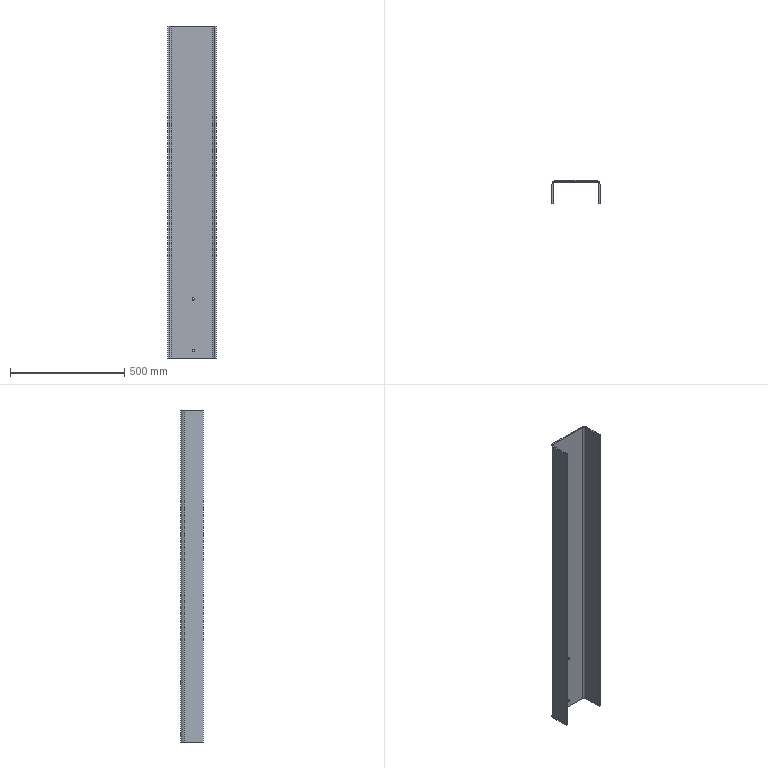Part | STEP file | _20001 | 1 solid | 18 faces | box 210 x 100 x 1450 mm | volume 3332053 mm3 | plane 10 | cylinder 8 | commonest cylinder face diameters 10.8 x4 18 x2 34 x2
STEP:
#1=CARTESIAN_POINT('',(10.9,0.,-467.));
#2=VERTEX_POINT('',#1);
#3=CARTESIAN_POINT('',(10.9,-6.,-467.));
#4=VERTEX_POINT('',#3);
#5=CARTESIAN_POINT('',(10.9,0.,-467.));
#6=DIRECTION('',(0.,-1.,0.));
#7=VECTOR('',#6,1000.);
#8=LINE('',#5,#7);
#9=EDGE_CURVE('',#2,#4,#8,.T.);
#10=ORIENTED_EDGE('',*,*,#9,.F.);
#11=CARTESIAN_POINT('',(0.1,0.,-467.));
#12=VERTEX_POINT('',#11);
#13=CARTESIAN_POINT('',(5.5,0.,-467.));
#14=DIRECTION('',(0.,-1.,0.));
#15=DIRECTION('',(-1.,0.,0.));
#16=AXIS2_PLACEMENT_3D('',#13,#14,#15);
#17=CIRCLE('',#16,5.4);
#18=EDGE_CURVE('',#12,#2,#17,.T.);
#19=ORIENTED_EDGE('',*,*,#18,.F.);
#20=CARTESIAN_POINT('',(0.1,-6.,-467.));
#21=VERTEX_POINT('',#20);
#22=CARTESIAN_POINT('',(0.1,0.,-467.));
#23=DIRECTION('',(0.,-1.,0.));
#24=VECTOR('',#23,1000.);
#25=LINE('',#22,#24);
#26=EDGE_CURVE('',#12,#21,#25,.T.);
#27=ORIENTED_EDGE('',*,*,#26,.T.);
#28=CARTESIAN_POINT('',(5.5,-6.,-467.));
#29=DIRECTION('',(0.,1.,0.));
#30=DIRECTION('',(1.,0.,0.));
#31=AXIS2_PLACEMENT_3D('',#28,#29,#30);
#32=CIRCLE('',#31,5.4);
#33=EDGE_CURVE('',#4,#21,#32,.T.);
#34=ORIENTED_EDGE('',*,*,#33,.F.);
#35=EDGE_LOOP('',(#10,#19,#27,#34));
#36=FACE_OUTER_BOUND('',#35,.T.);
#37=CARTESIAN_POINT('',(5.5,-10.,-467.));
#38=DIRECTION('',(0.,1.,0.));
#39=DIRECTION('',(-1.,0.,0.));
#40=AXIS2_PLACEMENT_3D('',#37,#38,#39);
#41=CYLINDRICAL_SURFACE('',#40,5.4);
#42=ADVANCED_FACE('',(#36),#41,.F.);
#43=CARTESIAN_POINT('',(5.5,-6.,-467.));
#44=DIRECTION('',(0.,1.,0.));
#45=DIRECTION('',(-1.,0.,0.));
#46=AXIS2_PLACEMENT_3D('',#43,#44,#45);
#47=CIRCLE('',#46,5.4);
#48=EDGE_CURVE('',#21,#4,#47,.T.);
#49=ORIENTED_EDGE('',*,*,#48,.F.);
#50=ORIENTED_EDGE('',*,*,#26,.F.);
#51=CARTESIAN_POINT('',(5.5,0.,-467.));
#52=DIRECTION('',(0.,-1.,0.));
#53=DIRECTION('',(1.,0.,0.));
#54=AXIS2_PLACEMENT_3D('',#51,#52,#53);
#55=CIRCLE('',#54,5.4);
#56=EDGE_CURVE('',#2,#12,#55,.T.);
#57=ORIENTED_EDGE('',*,*,#56,.F.);
#58=ORIENTED_EDGE('',*,*,#9,.T.);
#59=EDGE_LOOP('',(#49,#50,#57,#58));
#60=FACE_OUTER_BOUND('',#59,.T.);
#61=CARTESIAN_POINT('',(5.5,-10.,-467.));
#62=DIRECTION('',(0.,1.,0.));
#63=DIRECTION('',(-1.,0.,0.));
#64=AXIS2_PLACEMENT_3D('',#61,#62,#63);
#65=CYLINDRICAL_SURFACE('',#64,5.4);
#66=ADVANCED_FACE('',(#60),#65,.F.);
#67=CARTESIAN_POINT('',(88.,0.,-725.));
#68=VERTEX_POINT('',#67);
#69=CARTESIAN_POINT('',(88.,0.,725.));
#70=VERTEX_POINT('',#69);
#71=CARTESIAN_POINT('',(88.,0.,-725.));
#72=DIRECTION('',(0.,0.,1.));
#73=VECTOR('',#72,1000.);
#74=LINE('',#71,#73);
#75=EDGE_CURVE('',#68,#70,#74,.T.);
#76=ORIENTED_EDGE('',*,*,#75,.T.);
#77=CARTESIAN_POINT('',(105.,-17.,725.));
#78=VERTEX_POINT('',#77);
#79=CARTESIAN_POINT('',(88.,-17.,725.));
#80=DIRECTION('',(0.,0.,1.));
#81=DIRECTION('',(1.,0.,0.));
#82=AXIS2_PLACEMENT_3D('',#79,#80,#81);
#83=CIRCLE('',#82,17.);
#84=EDGE_CURVE('',#78,#70,#83,.T.);
#85=ORIENTED_EDGE('',*,*,#84,.F.);
#86=CARTESIAN_POINT('',(105.,-17.,-725.));
#87=VERTEX_POINT('',#86);
#88=CARTESIAN_POINT('',(105.,-17.,725.));
#89=DIRECTION('',(0.,0.,-1.));
#90=VECTOR('',#89,1000.);
#91=LINE('',#88,#90);
#92=EDGE_CURVE('',#78,#87,#91,.T.);
#93=ORIENTED_EDGE('',*,*,#92,.T.);
#94=CARTESIAN_POINT('',(88.,-17.,-725.));
#95=DIRECTION('',(0.,0.,-1.));
#96=DIRECTION('',(0.,1.,0.));
#97=AXIS2_PLACEMENT_3D('',#94,#95,#96);
#98=CIRCLE('',#97,17.);
#99=EDGE_CURVE('',#68,#87,#98,.T.);
#100=ORIENTED_EDGE('',*,*,#99,.F.);
#101=EDGE_LOOP('',(#76,#85,#93,#100));
#102=FACE_OUTER_BOUND('',#101,.T.);
#103=CARTESIAN_POINT('',(88.,-17.,725.));
#104=DIRECTION('',(0.,0.,-1.));
#105=DIRECTION('',(-1.,0.,0.));
#106=AXIS2_PLACEMENT_3D('',#103,#104,#105);
#107=CYLINDRICAL_SURFACE('',#106,17.);
#108=ADVANCED_FACE('',(#102),#107,.T.);
#109=ORIENTED_EDGE('',*,*,#92,.F.);
#110=CARTESIAN_POINT('',(105.,-100.,725.));
#111=VERTEX_POINT('',#110);
#112=CARTESIAN_POINT('',(105.,-17.,725.));
#113=DIRECTION('',(0.,-1.,0.));
#114=VECTOR('',#113,1000.);
#115=LINE('',#112,#114);
#116=EDGE_CURVE('',#78,#111,#115,.T.);
#117=ORIENTED_EDGE('',*,*,#116,.T.);
#118=CARTESIAN_POINT('',(105.,-100.,-725.));
#119=VERTEX_POINT('',#118);
#120=CARTESIAN_POINT('',(105.,-100.,-725.));
#121=DIRECTION('',(0.,0.,1.));
#122=VECTOR('',#121,1000.);
#123=LINE('',#120,#122);
#124=EDGE_CURVE('',#119,#111,#123,.T.);
#125=ORIENTED_EDGE('',*,*,#124,.F.);
#126=CARTESIAN_POINT('',(105.,-17.,-725.));
#127=DIRECTION('',(0.,-1.,0.));
#128=VECTOR('',#127,1000.);
#129=LINE('',#126,#128);
#130=EDGE_CURVE('',#87,#119,#129,.T.);
#131=ORIENTED_EDGE('',*,*,#130,.F.);
#132=EDGE_LOOP('',(#109,#117,#125,#131));
#133=FACE_OUTER_BOUND('',#132,.T.);
#134=CARTESIAN_POINT('',(105.,0.,725.));
#135=DIRECTION('',(-1.,0.,0.));
#136=DIRECTION('',(0.,0.,1.));
#137=AXIS2_PLACEMENT_3D('',#134,#135,#136);
#138=PLANE('',#137);
#139=ADVANCED_FACE('',(#133),#138,.F.);
#140=ORIENTED_EDGE('',*,*,#124,.T.);
#141=CARTESIAN_POINT('',(99.,-100.,725.));
#142=VERTEX_POINT('',#141);
#143=CARTESIAN_POINT('',(99.,-100.,725.));
#144=DIRECTION('',(1.,0.,0.));
#145=VECTOR('',#144,1000.);
#146=LINE('',#143,#145);
#147=EDGE_CURVE('',#142,#111,#146,.T.);
#148=ORIENTED_EDGE('',*,*,#147,.F.);
#149=CARTESIAN_POINT('',(99.,-100.,-725.));
#150=VERTEX_POINT('',#149);
#151=CARTESIAN_POINT('',(99.,-100.,-725.));
#152=DIRECTION('',(0.,0.,1.));
#153=VECTOR('',#152,1000.);
#154=LINE('',#151,#153);
#155=EDGE_CURVE('',#150,#142,#154,.T.);
#156=ORIENTED_EDGE('',*,*,#155,.F.);
#157=CARTESIAN_POINT('',(99.,-100.,-725.));
#158=DIRECTION('',(1.,0.,0.));
#159=VECTOR('',#158,1000.);
#160=LINE('',#157,#159);
#161=EDGE_CURVE('',#150,#119,#160,.T.);
#162=ORIENTED_EDGE('',*,*,#161,.T.);
#163=EDGE_LOOP('',(#140,#148,#156,#162));
#164=FACE_OUTER_BOUND('',#163,.T.);
#165=CARTESIAN_POINT('',(105.,-100.,725.));
#166=DIRECTION('',(0.,-1.,0.));
#167=DIRECTION('',(0.,0.,-1.));
#168=AXIS2_PLACEMENT_3D('',#165,#166,#167);
#169=PLANE('',#168);
#170=ADVANCED_FACE('',(#164),#169,.T.);
#171=CARTESIAN_POINT('',(99.,-15.,-725.));
#172=VERTEX_POINT('',#171);
#173=CARTESIAN_POINT('',(99.,-15.,-725.));
#174=DIRECTION('',(0.,-1.,0.));
#175=VECTOR('',#174,1000.);
#176=LINE('',#173,#175);
#177=EDGE_CURVE('',#172,#150,#176,.T.);
#178=ORIENTED_EDGE('',*,*,#177,.T.);
#179=ORIENTED_EDGE('',*,*,#155,.T.);
#180=CARTESIAN_POINT('',(99.,-15.,725.));
#181=VERTEX_POINT('',#180);
#182=CARTESIAN_POINT('',(99.,-100.,725.));
#183=DIRECTION('',(0.,1.,0.));
#184=VECTOR('',#183,1000.);
#185=LINE('',#182,#184);
#186=EDGE_CURVE('',#142,#181,#185,.T.);
#187=ORIENTED_EDGE('',*,*,#186,.T.);
#188=CARTESIAN_POINT('',(99.,-15.,-725.));
#189=DIRECTION('',(0.,0.,1.));
#190=VECTOR('',#189,1000.);
#191=LINE('',#188,#190);
#192=EDGE_CURVE('',#172,#181,#191,.T.);
#193=ORIENTED_EDGE('',*,*,#192,.F.);
#194=EDGE_LOOP('',(#178,#179,#187,#193));
#195=FACE_OUTER_BOUND('',#194,.T.);
#196=CARTESIAN_POINT('',(99.,0.,725.));
#197=DIRECTION('',(-1.,0.,0.));
#198=DIRECTION('',(0.,0.,1.));
#199=AXIS2_PLACEMENT_3D('',#196,#197,#198);
#200=PLANE('',#199);
#201=ADVANCED_FACE('',(#195),#200,.T.);
#202=CARTESIAN_POINT('',(90.,-6.,-725.));
#203=VERTEX_POINT('',#202);
#204=CARTESIAN_POINT('',(90.,-15.,-725.));
#205=DIRECTION('',(0.,0.,1.));
#206=DIRECTION('',(1.,0.,0.));
#207=AXIS2_PLACEMENT_3D('',#204,#205,#206);
#208=CIRCLE('',#207,9.);
#209=EDGE_CURVE('',#172,#203,#208,.T.);
#210=ORIENTED_EDGE('',*,*,#209,.F.);
#211=ORIENTED_EDGE('',*,*,#192,.T.);
#212=CARTESIAN_POINT('',(90.,-6.,725.));
#213=VERTEX_POINT('',#212);
#214=CARTESIAN_POINT('',(90.,-15.,725.));
#215=DIRECTION('',(0.,0.,-1.));
#216=DIRECTION('',(0.,1.,0.));
#217=AXIS2_PLACEMENT_3D('',#214,#215,#216);
#218=CIRCLE('',#217,9.);
#219=EDGE_CURVE('',#213,#181,#218,.T.);
#220=ORIENTED_EDGE('',*,*,#219,.F.);
#221=CARTESIAN_POINT('',(90.,-6.,-725.));
#222=DIRECTION('',(0.,0.,1.));
#223=VECTOR('',#222,1000.);
#224=LINE('',#221,#223);
#225=EDGE_CURVE('',#203,#213,#224,.T.);
#226=ORIENTED_EDGE('',*,*,#225,.F.);
#227=EDGE_LOOP('',(#210,#211,#220,#226));
#228=FACE_OUTER_BOUND('',#227,.T.);
#229=CARTESIAN_POINT('',(90.,-15.,-2615.22));
#230=DIRECTION('',(0.,0.,1.));
#231=DIRECTION('',(1.,0.,0.));
#232=AXIS2_PLACEMENT_3D('',#229,#230,#231);
#233=CYLINDRICAL_SURFACE('',#232,9.);
#234=ADVANCED_FACE('',(#228),#233,.F.);
#235=CARTESIAN_POINT('',(-105.,-17.,-725.));
#236=VERTEX_POINT('',#235);
#237=CARTESIAN_POINT('',(-105.,-17.,725.));
#238=VERTEX_POINT('',#237);
#239=CARTESIAN_POINT('',(-105.,-17.,-725.));
#240=DIRECTION('',(0.,0.,1.));
#241=VECTOR('',#240,1000.);
#242=LINE('',#239,#241);
#243=EDGE_CURVE('',#236,#238,#242,.T.);
#244=ORIENTED_EDGE('',*,*,#243,.T.);
#245=CARTESIAN_POINT('',(-88.,0.,725.));
#246=VERTEX_POINT('',#245);
#247=CARTESIAN_POINT('',(-88.,-17.,725.));
#248=DIRECTION('',(0.,0.,1.));
#249=DIRECTION('',(0.,1.,0.));
#250=AXIS2_PLACEMENT_3D('',#247,#248,#249);
#251=CIRCLE('',#250,17.);
#252=EDGE_CURVE('',#246,#238,#251,.T.);
#253=ORIENTED_EDGE('',*,*,#252,.F.);
#254=CARTESIAN_POINT('',(-88.,0.,-725.));
#255=VERTEX_POINT('',#254);
#256=CARTESIAN_POINT('',(-88.,0.,725.));
#257=DIRECTION('',(0.,0.,-1.));
#258=VECTOR('',#257,1000.);
#259=LINE('',#256,#258);
#260=EDGE_CURVE('',#246,#255,#259,.T.);
#261=ORIENTED_EDGE('',*,*,#260,.T.);
#262=CARTESIAN_POINT('',(-88.,-17.,-725.));
#263=DIRECTION('',(0.,0.,-1.));
#264=DIRECTION('',(-1.,0.,0.));
#265=AXIS2_PLACEMENT_3D('',#262,#263,#264);
#266=CIRCLE('',#265,17.);
#267=EDGE_CURVE('',#236,#255,#266,.T.);
#268=ORIENTED_EDGE('',*,*,#267,.F.);
#269=EDGE_LOOP('',(#244,#253,#261,#268));
#270=FACE_OUTER_BOUND('',#269,.T.);
#271=CARTESIAN_POINT('',(-88.,-17.,725.));
#272=DIRECTION('',(0.,0.,-1.));
#273=DIRECTION('',(-1.,0.,0.));
#274=AXIS2_PLACEMENT_3D('',#271,#272,#273);
#275=CYLINDRICAL_SURFACE('',#274,17.);
#276=ADVANCED_FACE('',(#270),#275,.T.);
#277=CARTESIAN_POINT('',(-105.,-100.,-725.));
#278=VERTEX_POINT('',#277);
#279=CARTESIAN_POINT('',(-105.,-100.,725.));
#280=VERTEX_POINT('',#279);
#281=CARTESIAN_POINT('',(-105.,-100.,-725.));
#282=DIRECTION('',(0.,0.,1.));
#283=VECTOR('',#282,1000.);
#284=LINE('',#281,#283);
#285=EDGE_CURVE('',#278,#280,#284,.T.);
#286=ORIENTED_EDGE('',*,*,#285,.T.);
#287=CARTESIAN_POINT('',(-105.,-100.,725.));
#288=DIRECTION('',(0.,1.,0.));
#289=VECTOR('',#288,1000.);
#290=LINE('',#287,#289);
#291=EDGE_CURVE('',#280,#238,#290,.T.);
#292=ORIENTED_EDGE('',*,*,#291,.T.);
#293=ORIENTED_EDGE('',*,*,#243,.F.);
#294=CARTESIAN_POINT('',(-105.,-100.,-725.));
#295=DIRECTION('',(0.,1.,0.));
#296=VECTOR('',#295,1000.);
#297=LINE('',#294,#296);
#298=EDGE_CURVE('',#278,#236,#297,.T.);
#299=ORIENTED_EDGE('',*,*,#298,.F.);
#300=EDGE_LOOP('',(#286,#292,#293,#299));
#301=FACE_OUTER_BOUND('',#300,.T.);
#302=CARTESIAN_POINT('',(-105.,0.,725.));
#303=DIRECTION('',(1.,0.,0.));
#304=DIRECTION('',(0.,1.,0.));
#305=AXIS2_PLACEMENT_3D('',#302,#303,#304);
#306=PLANE('',#305);
#307=ADVANCED_FACE('',(#301),#306,.F.);
#308=CARTESIAN_POINT('',(-99.,-100.,-725.));
#309=VERTEX_POINT('',#308);
#310=CARTESIAN_POINT('',(-99.,-100.,725.));
#311=VERTEX_POINT('',#310);
#312=CARTESIAN_POINT('',(-99.,-100.,-725.));
#313=DIRECTION('',(0.,0.,1.));
#314=VECTOR('',#313,1000.);
#315=LINE('',#312,#314);
#316=EDGE_CURVE('',#309,#311,#315,.T.);
#317=ORIENTED_EDGE('',*,*,#316,.T.);
#318=CARTESIAN_POINT('',(-105.,-100.,725.));
#319=DIRECTION('',(1.,0.,0.));
#320=VECTOR('',#319,1000.);
#321=LINE('',#318,#320);
#322=EDGE_CURVE('',#280,#311,#321,.T.);
#323=ORIENTED_EDGE('',*,*,#322,.F.);
#324=ORIENTED_EDGE('',*,*,#285,.F.);
#325=CARTESIAN_POINT('',(-105.,-100.,-725.));
#326=DIRECTION('',(1.,0.,0.));
#327=VECTOR('',#326,1000.);
#328=LINE('',#325,#327);
#329=EDGE_CURVE('',#278,#309,#328,.T.);
#330=ORIENTED_EDGE('',*,*,#329,.T.);
#331=EDGE_LOOP('',(#317,#323,#324,#330));
#332=FACE_OUTER_BOUND('',#331,.T.);
#333=CARTESIAN_POINT('',(-97.,-100.,725.));
#334=DIRECTION('',(0.,-1.,0.));
#335=DIRECTION('',(0.,0.,-1.));
#336=AXIS2_PLACEMENT_3D('',#333,#334,#335);
#337=PLANE('',#336);
#338=ADVANCED_FACE('',(#332),#337,.T.);
#339=CARTESIAN_POINT('',(-90.,-6.,-725.));
#340=VERTEX_POINT('',#339);
#341=CARTESIAN_POINT('',(-99.,-15.,-725.));
#342=VERTEX_POINT('',#341);
#343=CARTESIAN_POINT('',(-90.,-15.,-725.));
#344=DIRECTION('',(0.,0.,1.));
#345=DIRECTION('',(0.,1.,0.));
#346=AXIS2_PLACEMENT_3D('',#343,#344,#345);
#347=CIRCLE('',#346,9.);
#348=EDGE_CURVE('',#340,#342,#347,.T.);
#349=ORIENTED_EDGE('',*,*,#348,.F.);
#350=CARTESIAN_POINT('',(-90.,-6.,725.));
#351=VERTEX_POINT('',#350);
#352=CARTESIAN_POINT('',(-90.,-6.,-725.));
#353=DIRECTION('',(0.,0.,1.));
#354=VECTOR('',#353,1000.);
#355=LINE('',#352,#354);
#356=EDGE_CURVE('',#340,#351,#355,.T.);
#357=ORIENTED_EDGE('',*,*,#356,.T.);
#358=CARTESIAN_POINT('',(-99.,-15.,725.));
#359=VERTEX_POINT('',#358);
#360=CARTESIAN_POINT('',(-90.,-15.,725.));
#361=DIRECTION('',(0.,0.,-1.));
#362=DIRECTION('',(-1.,0.,0.));
#363=AXIS2_PLACEMENT_3D('',#360,#361,#362);
#364=CIRCLE('',#363,9.);
#365=EDGE_CURVE('',#359,#351,#364,.T.);
#366=ORIENTED_EDGE('',*,*,#365,.F.);
#367=CARTESIAN_POINT('',(-99.,-15.,-725.));
#368=DIRECTION('',(0.,0.,1.));
#369=VECTOR('',#368,1000.);
#370=LINE('',#367,#369);
#371=EDGE_CURVE('',#342,#359,#370,.T.);
#372=ORIENTED_EDGE('',*,*,#371,.F.);
#373=EDGE_LOOP('',(#349,#357,#366,#372));
#374=FACE_OUTER_BOUND('',#373,.T.);
#375=CARTESIAN_POINT('',(-90.,-15.,-2615.22));
#376=DIRECTION('',(0.,0.,1.));
#377=DIRECTION('',(0.,1.,0.));
#378=AXIS2_PLACEMENT_3D('',#375,#376,#377);
#379=CYLINDRICAL_SURFACE('',#378,9.);
#380=ADVANCED_FACE('',(#374),#379,.F.);
#381=CARTESIAN_POINT('',(-99.,-15.,725.));
#382=DIRECTION('',(0.,-1.,0.));
#383=VECTOR('',#382,1000.);
#384=LINE('',#381,#383);
#385=EDGE_CURVE('',#359,#311,#384,.T.);
#386=ORIENTED_EDGE('',*,*,#385,.T.);
#387=ORIENTED_EDGE('',*,*,#316,.F.);
#388=CARTESIAN_POINT('',(-99.,-100.,-725.));
#389=DIRECTION('',(0.,1.,0.));
#390=VECTOR('',#389,1000.);
#391=LINE('',#388,#390);
#392=EDGE_CURVE('',#309,#342,#391,.T.);
#393=ORIENTED_EDGE('',*,*,#392,.T.);
#394=ORIENTED_EDGE('',*,*,#371,.T.);
#395=EDGE_LOOP('',(#386,#387,#393,#394));
#396=FACE_OUTER_BOUND('',#395,.T.);
#397=CARTESIAN_POINT('',(-99.,0.,725.));
#398=DIRECTION('',(1.,0.,0.));
#399=DIRECTION('',(0.,1.,0.));
#400=AXIS2_PLACEMENT_3D('',#397,#398,#399);
#401=PLANE('',#400);
#402=ADVANCED_FACE('',(#396),#401,.T.);
#403=ORIENTED_EDGE('',*,*,#329,.F.);
#404=ORIENTED_EDGE('',*,*,#298,.T.);
#405=ORIENTED_EDGE('',*,*,#267,.T.);
#406=CARTESIAN_POINT('',(-88.,0.,-725.));
#407=DIRECTION('',(1.,0.,0.));
#408=VECTOR('',#407,1000.);
#409=LINE('',#406,#408);
#410=EDGE_CURVE('',#255,#68,#409,.T.);
#411=ORIENTED_EDGE('',*,*,#410,.T.);
#412=ORIENTED_EDGE('',*,*,#99,.T.);
#413=ORIENTED_EDGE('',*,*,#130,.T.);
#414=ORIENTED_EDGE('',*,*,#161,.F.);
#415=ORIENTED_EDGE('',*,*,#177,.F.);
#416=ORIENTED_EDGE('',*,*,#209,.T.);
#417=CARTESIAN_POINT('',(-90.,-6.,-725.));
#418=DIRECTION('',(1.,0.,0.));
#419=VECTOR('',#418,1000.);
#420=LINE('',#417,#419);
#421=EDGE_CURVE('',#340,#203,#420,.T.);
#422=ORIENTED_EDGE('',*,*,#421,.F.);
#423=ORIENTED_EDGE('',*,*,#348,.T.);
#424=ORIENTED_EDGE('',*,*,#392,.F.);
#425=EDGE_LOOP('',(#403,#404,#405,#411,#412,#413,#414,#415,#416,#422,#423,#424));
#426=FACE_OUTER_BOUND('',#425,.T.);
#427=CARTESIAN_POINT('',(97.,-17.,-725.));
#428=DIRECTION('',(0.,0.,-1.));
#429=DIRECTION('',(0.,-1.,0.));
#430=AXIS2_PLACEMENT_3D('',#427,#428,#429);
#431=PLANE('',#430);
#432=ADVANCED_FACE('',(#426),#431,.T.);
#433=ORIENTED_EDGE('',*,*,#18,.T.);
#434=ORIENTED_EDGE('',*,*,#56,.T.);
#435=EDGE_LOOP('',(#433,#434));
#436=FACE_BOUND('',#435,.T.);
#437=CARTESIAN_POINT('',(0.1,0.,-693.));
#438=VERTEX_POINT('',#437);
#439=CARTESIAN_POINT('',(10.9,0.,-693.));
#440=VERTEX_POINT('',#439);
#441=CARTESIAN_POINT('',(5.5,0.,-693.));
#442=DIRECTION('',(0.,-1.,0.));
#443=DIRECTION('',(-1.,0.,0.));
#444=AXIS2_PLACEMENT_3D('',#441,#442,#443);
#445=CIRCLE('',#444,5.4);
#446=EDGE_CURVE('',#438,#440,#445,.T.);
#447=ORIENTED_EDGE('',*,*,#446,.T.);
#448=CARTESIAN_POINT('',(5.5,0.,-693.));
#449=DIRECTION('',(0.,-1.,0.));
#450=DIRECTION('',(1.,0.,0.));
#451=AXIS2_PLACEMENT_3D('',#448,#449,#450);
#452=CIRCLE('',#451,5.4);
#453=EDGE_CURVE('',#440,#438,#452,.T.);
#454=ORIENTED_EDGE('',*,*,#453,.T.);
#455=EDGE_LOOP('',(#447,#454));
#456=FACE_BOUND('',#455,.T.);
#457=ORIENTED_EDGE('',*,*,#260,.F.);
#458=CARTESIAN_POINT('',(-88.,0.,725.));
#459=DIRECTION('',(1.,0.,0.));
#460=VECTOR('',#459,1000.);
#461=LINE('',#458,#460);
#462=EDGE_CURVE('',#246,#70,#461,.T.);
#463=ORIENTED_EDGE('',*,*,#462,.T.);
#464=ORIENTED_EDGE('',*,*,#75,.F.);
#465=ORIENTED_EDGE('',*,*,#410,.F.);
#466=EDGE_LOOP('',(#457,#463,#464,#465));
#467=FACE_OUTER_BOUND('',#466,.T.);
#468=CARTESIAN_POINT('',(-105.,0.,725.));
#469=DIRECTION('',(0.,-1.,0.));
#470=DIRECTION('',(0.,0.,-1.));
#471=AXIS2_PLACEMENT_3D('',#468,#469,#470);
#472=PLANE('',#471);
#473=ADVANCED_FACE('',(#436,#456,#467),#472,.F.);
#474=CARTESIAN_POINT('',(0.1,-6.,-693.));
#475=VERTEX_POINT('',#474);
#476=CARTESIAN_POINT('',(10.9,-6.,-693.));
#477=VERTEX_POINT('',#476);
#478=CARTESIAN_POINT('',(5.5,-6.,-693.));
#479=DIRECTION('',(0.,1.,0.));
#480=DIRECTION('',(-1.,0.,0.));
#481=AXIS2_PLACEMENT_3D('',#478,#479,#480);
#482=CIRCLE('',#481,5.4);
#483=EDGE_CURVE('',#475,#477,#482,.T.);
#484=ORIENTED_EDGE('',*,*,#483,.F.);
#485=CARTESIAN_POINT('',(0.1,0.,-693.));
#486=DIRECTION('',(0.,-1.,0.));
#487=VECTOR('',#486,1000.);
#488=LINE('',#485,#487);
#489=EDGE_CURVE('',#438,#475,#488,.T.);
#490=ORIENTED_EDGE('',*,*,#489,.F.);
#491=ORIENTED_EDGE('',*,*,#453,.F.);
#492=CARTESIAN_POINT('',(10.9,0.,-693.));
#493=DIRECTION('',(0.,-1.,0.));
#494=VECTOR('',#493,1000.);
#495=LINE('',#492,#494);
#496=EDGE_CURVE('',#440,#477,#495,.T.);
#497=ORIENTED_EDGE('',*,*,#496,.T.);
#498=EDGE_LOOP('',(#484,#490,#491,#497));
#499=FACE_OUTER_BOUND('',#498,.T.);
#500=CARTESIAN_POINT('',(5.5,-10.,-693.));
#501=DIRECTION('',(0.,1.,0.));
#502=DIRECTION('',(-1.,0.,0.));
#503=AXIS2_PLACEMENT_3D('',#500,#501,#502);
#504=CYLINDRICAL_SURFACE('',#503,5.4);
#505=ADVANCED_FACE('',(#499),#504,.F.);
#506=ORIENTED_EDGE('',*,*,#496,.F.);
#507=ORIENTED_EDGE('',*,*,#446,.F.);
#508=ORIENTED_EDGE('',*,*,#489,.T.);
#509=CARTESIAN_POINT('',(5.5,-6.,-693.));
#510=DIRECTION('',(0.,1.,0.));
#511=DIRECTION('',(1.,0.,0.));
#512=AXIS2_PLACEMENT_3D('',#509,#510,#511);
#513=CIRCLE('',#512,5.4);
#514=EDGE_CURVE('',#477,#475,#513,.T.);
#515=ORIENTED_EDGE('',*,*,#514,.F.);
#516=EDGE_LOOP('',(#506,#507,#508,#515));
#517=FACE_OUTER_BOUND('',#516,.T.);
#518=CARTESIAN_POINT('',(5.5,-10.,-693.));
#519=DIRECTION('',(0.,1.,0.));
#520=DIRECTION('',(-1.,0.,0.));
#521=AXIS2_PLACEMENT_3D('',#518,#519,#520);
#522=CYLINDRICAL_SURFACE('',#521,5.4);
#523=ADVANCED_FACE('',(#517),#522,.F.);
#524=ORIENTED_EDGE('',*,*,#483,.T.);
#525=ORIENTED_EDGE('',*,*,#514,.T.);
#526=EDGE_LOOP('',(#524,#525));
#527=FACE_BOUND('',#526,.T.);
#528=ORIENTED_EDGE('',*,*,#48,.T.);
#529=ORIENTED_EDGE('',*,*,#33,.T.);
#530=EDGE_LOOP('',(#528,#529));
#531=FACE_BOUND('',#530,.T.);
#532=CARTESIAN_POINT('',(90.,-6.,725.));
#533=DIRECTION('',(-1.,0.,0.));
#534=VECTOR('',#533,1000.);
#535=LINE('',#532,#534);
#536=EDGE_CURVE('',#213,#351,#535,.T.);
#537=ORIENTED_EDGE('',*,*,#536,.T.);
#538=ORIENTED_EDGE('',*,*,#356,.F.);
#539=ORIENTED_EDGE('',*,*,#421,.T.);
#540=ORIENTED_EDGE('',*,*,#225,.T.);
#541=EDGE_LOOP('',(#537,#538,#539,#540));
#542=FACE_OUTER_BOUND('',#541,.T.);
#543=CARTESIAN_POINT('',(-105.,-6.,725.));
#544=DIRECTION('',(0.,-1.,0.));
#545=DIRECTION('',(0.,0.,-1.));
#546=AXIS2_PLACEMENT_3D('',#543,#544,#545);
#547=PLANE('',#546);
#548=ADVANCED_FACE('',(#527,#531,#542),#547,.T.);
#549=ORIENTED_EDGE('',*,*,#219,.T.);
#550=ORIENTED_EDGE('',*,*,#186,.F.);
#551=ORIENTED_EDGE('',*,*,#147,.T.);
#552=ORIENTED_EDGE('',*,*,#116,.F.);
#553=ORIENTED_EDGE('',*,*,#84,.T.);
#554=ORIENTED_EDGE('',*,*,#462,.F.);
#555=ORIENTED_EDGE('',*,*,#252,.T.);
#556=ORIENTED_EDGE('',*,*,#291,.F.);
#557=ORIENTED_EDGE('',*,*,#322,.T.);
#558=ORIENTED_EDGE('',*,*,#385,.F.);
#559=ORIENTED_EDGE('',*,*,#365,.T.);
#560=ORIENTED_EDGE('',*,*,#536,.F.);
#561=EDGE_LOOP('',(#549,#550,#551,#552,#553,#554,#555,#556,#557,#558,#559,#560));
#562=FACE_OUTER_BOUND('',#561,.T.);
#563=CARTESIAN_POINT('',(105.,-17.,725.));
#564=DIRECTION('',(0.,0.,1.));
#565=DIRECTION('',(1.,0.,0.));
#566=AXIS2_PLACEMENT_3D('',#563,#564,#565);
#567=PLANE('',#566);
#568=ADVANCED_FACE('',(#562),#567,.T.);
#569=CLOSED_SHELL('',(#42,#66,#108,#139,#170,#201,#234,#276,#307,#338,#380,#402,#432,#473,#505,#523,#548,#568));
#570=MANIFOLD_SOLID_BREP('',#569);
#571=CARTESIAN_POINT('',(0.,0.,0.));
#572=DIRECTION('',(0.,0.,1.));
#573=DIRECTION('',(1.,0.,0.));
#574=AXIS2_PLACEMENT_3D('',#571,#572,#573);
#575=(LENGTH_UNIT()NAMED_UNIT(*)SI_UNIT(.MILLI.,.METRE.));
#576=UNCERTAINTY_MEASURE_WITH_UNIT(LENGTH_MEASURE(0.00001),#575,'','');
#577=(NAMED_UNIT(*)PLANE_ANGLE_UNIT()SI_UNIT($,.RADIAN.));
#578=(NAMED_UNIT(*)SI_UNIT($,.STERADIAN.)SOLID_ANGLE_UNIT());
#579=(GEOMETRIC_REPRESENTATION_CONTEXT(3)GLOBAL_UNCERTAINTY_ASSIGNED_CONTEXT((#576))GLOBAL_UNIT_ASSIGNED_CONTEXT((#575,#577,#578))REPRESENTATION_CONTEXT('',''));
#580=ADVANCED_BREP_SHAPE_REPRESENTATION('',(#570,#574),#579);